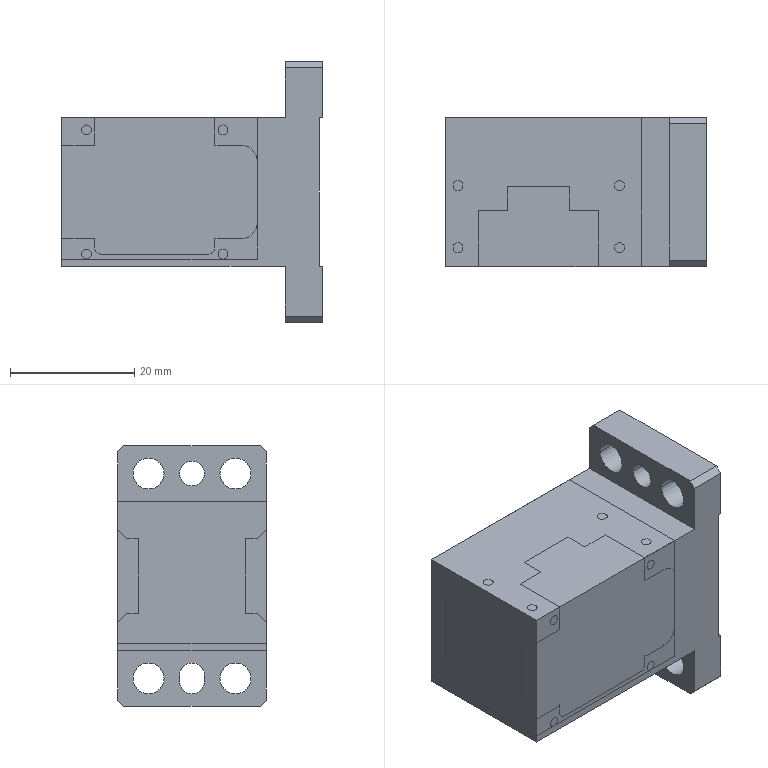NC program | NX | posted with a generic post | part box 42 x 24 x 42 mm
Lines 3952 to 4089 of 4089:
(CAVITY_MILL_COPY_1 , TOOL : D10JING)
N7890 T11 M6
N7892 G54
N7894 G17 G0 G90 X22.622 Y-18.809 B0. C0. S5000 M3
N7896 G43 Z30. H11
N7898 Z-13.
N7900 G94 G1 Z-14. F1000.
N7902 X21.866 Y-17.5
N7904 G3 X21. Y-17. R1.
N7906 G1 X-21.
N7908 G2 X-26. Y-12. R5.
N7910 G1 Y12.
N7912 G2 X-21. Y17. R5.
N7914 G1 X21.
N7916 G2 X26. Y12. R5.
N7918 G1 Y-12.
N7920 G2 X21. Y-17. R5.
N7922 G3 X20.134 Y-17.5 R1.
N7924 G1 X19.268 Y-19.
N7926 Z-13.
N7928 G0 Z30.
N7930 X22.622 Y-18.809
N7932 Z-27.
N7934 G1 Z-28.
N7936 X21.866 Y-17.5
N7938 G3 X21. Y-17. R1.
N7940 G1 X-21.
N7942 G2 X-26. Y-12. R5.
N7944 G1 Y12.
N7946 G2 X-21. Y17. R5.
N7948 G1 X21.
N7950 G2 X26. Y12. R5.
N7952 G1 Y-12.
N7954 G2 X21. Y-17. R5.
N7956 G3 X20.134 Y-17.5 R1.
N7958 G1 X19.268 Y-19.
N7960 Z-27.
N7962 G0 Z-11.
N7964 X22.622 Y-18.809
N7966 Z-41.
N7968 G1 Z-42.
N7970 X21.866 Y-17.5
N7972 G3 X21. Y-17. R1.
N7974 G1 X-21.
N7976 G2 X-26. Y-12. R5.
N7978 G1 Y12.
N7980 G2 X-21. Y17. R5.
N7982 G1 X21.
N7984 G2 X26. Y12. R5.
N7986 G1 Y-12.
N7988 G2 X21. Y-17. R5.
N7990 G3 X20.134 Y-17.5 R1.
N7992 G1 X19.268 Y-19.
N7994 Z-41.
N7996 G0 Z30.
(FLOOR_WALL_1_1 , TOOL : D10JING)
N7998 X23.463 Y19. S5500
N8000 Z-7.5
N8002 G1 Z-9. F1250.
N8004 X21.499 Y17.866
N8006 G3 X20.999 Y17. R1.
N8008 G1 Y-17.
N8010 X16.642
N8012 Y17.
N8014 X12.285
N8016 Y-17.
N8018 X7.928
N8020 Y17.
N8022 X3.571
N8024 Y-17.
N8026 X-0.786
N8028 Y17.
N8030 X-5.143
N8032 Y-17.
N8034 X-9.5
N8036 Y17.
N8038 G2 X-9. Y17.866 R1.
N8040 G1 X-7.036 Y19.
N8042 Z-7.5
N8044 G0 Z30.
N8046 X-7.536
N8048 Z-7.5
N8050 G1 Z-9.
N8052 X-9.5 Y17.866
N8054 G3 X-10. Y17. R1.
N8056 G1 Y-17.
N8058 G3 X-9.5 Y-17.866 R1.
N8060 G1 X-7.536 Y-19.
N8062 Z-7.5
N8064 G0 Z30.
N8066 M5
(PLANAR_MILL , TOOL : D6A45)
N8068 T07 M6
N8070 G54
N8072 G17 G0 G90 X-10.908 Y14.313 B0. C0. S7500 M3
N8074 G43 Z30. H7
N8076 Z-8.5
N8078 G94 G1 Z-10. F1250.
N8080 X-11.357 Y13.865
N8082 G3 X-11.618 Y12.9 R1.
N8084 G1 X20.9
N8086 G2 X21.9 Y11.9 R1.
N8088 G1 Y-11.9
N8090 G2 X20.9 Y-12.9 R1.
N8092 G1 X-11.618
N8094 G3 X-11.357 Y-13.865 R1.
N8096 G1 X-10.908 Y-14.313
N8098 Z-8.5
N8100 G0 Z30.
(PLANAR_MILL_COPY , TOOL : D6A45)
N8102 X-24.1 Y-1.27
N8104 Z-0.5
N8106 G1 Z-2.
N8108 X-23.4 Y-0.866
N8110 G3 X-22.9 Y0. R1.
N8112 G1 Y10.9
N8114 G2 X-20.9 Y12.9 R2.
N8116 G1 X-15.1
N8118 G2 X-13.1 Y10.9 R2.
N8120 G1 Y-10.9
N8122 G2 X-15.1 Y-12.9 R2.
N8124 G1 X-20.9
N8126 G2 X-22.9 Y-10.9 R2.
N8128 G1 Y0.
N8130 G3 X-23.4 Y0.866 R1.
N8132 G1 X-24.1 Y1.27
N8134 Z-0.5
N8136 G0 Z30.
N8138 M5
N8140 M2